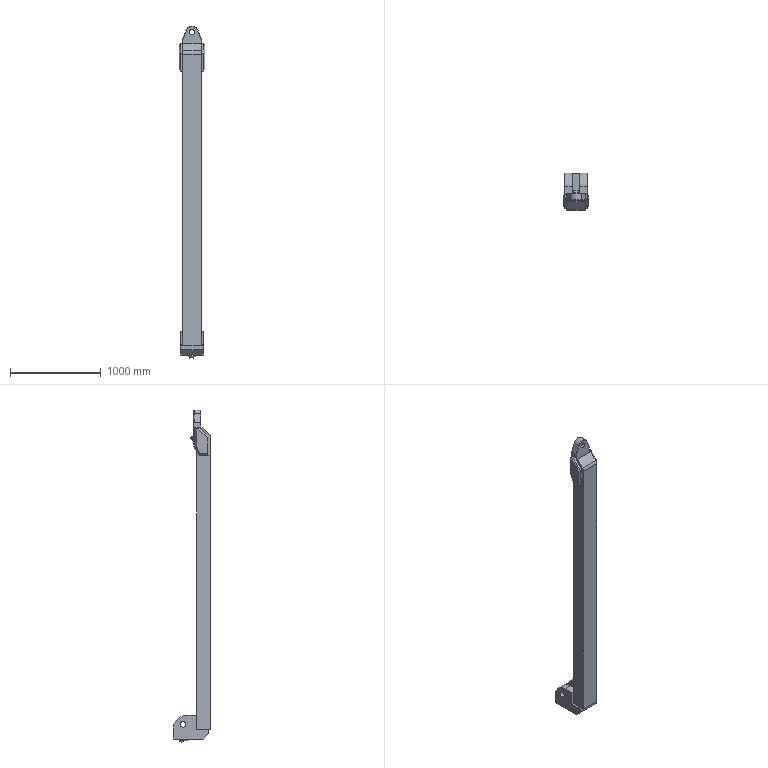Part | NX | features 推移杆 2 | 1 solid | 100 faces | box 283.14 x 415 x 3654 mm | volume 76372514 mm3 | plane 78 | cylinder 17 | torus 3 | cone 2 | commonest cylinder face diameters 17.3 x6 20 x2 40.9 x2 62 x2 300 x2 60 x1